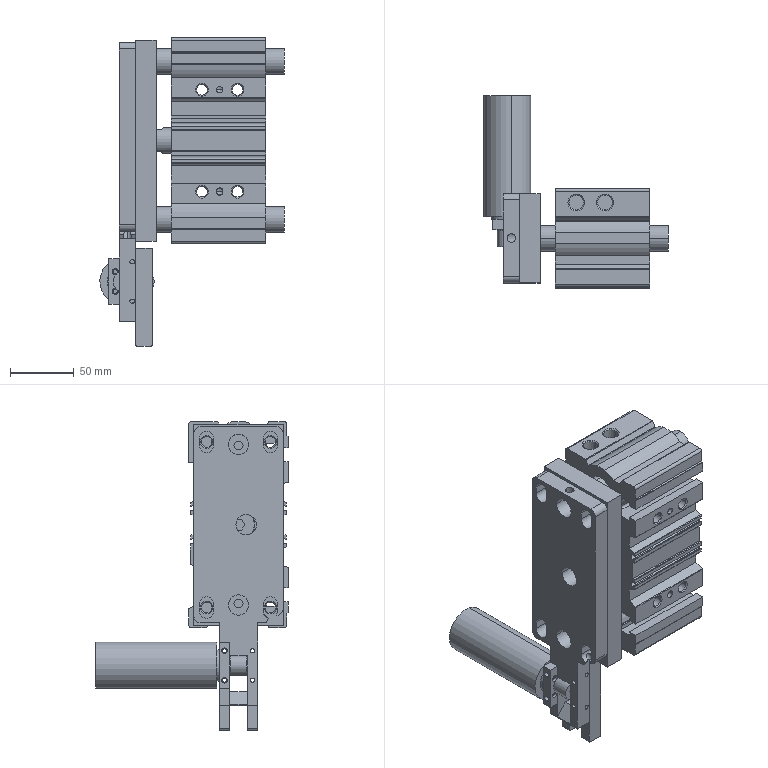Part | 11 solids | 602 faces | box 144.65 x 151 x 242.5 mm | volume 1151077 mm3 | cylinder 254 | plane 236 | cone 48 | sphere 48 | torus 16 | commonest cylinder face diameters 5 x40 8.376 x24 1 x22 11 x17 20 x16 4.2 x12